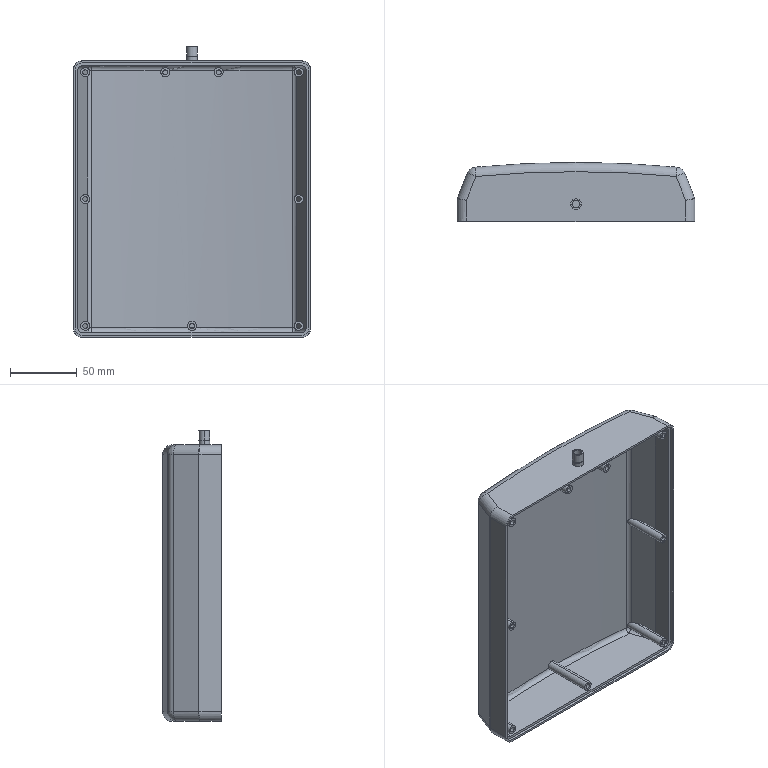Part | SolidWorks | features ICE 2, Extrusion 1, Fillet 1, Revolution 1, Shell 1 | 1 solid | 141 faces | box 178 x 44 x 217.6 mm | volume 217327 mm3 | cylinder 83 | plane 35 | torus 11 | sphere 8 | spline 4 | commonest cylinder face diameters 7 x20 3.8 x18 6.8 x18 14 x10 8 x4 11 x4